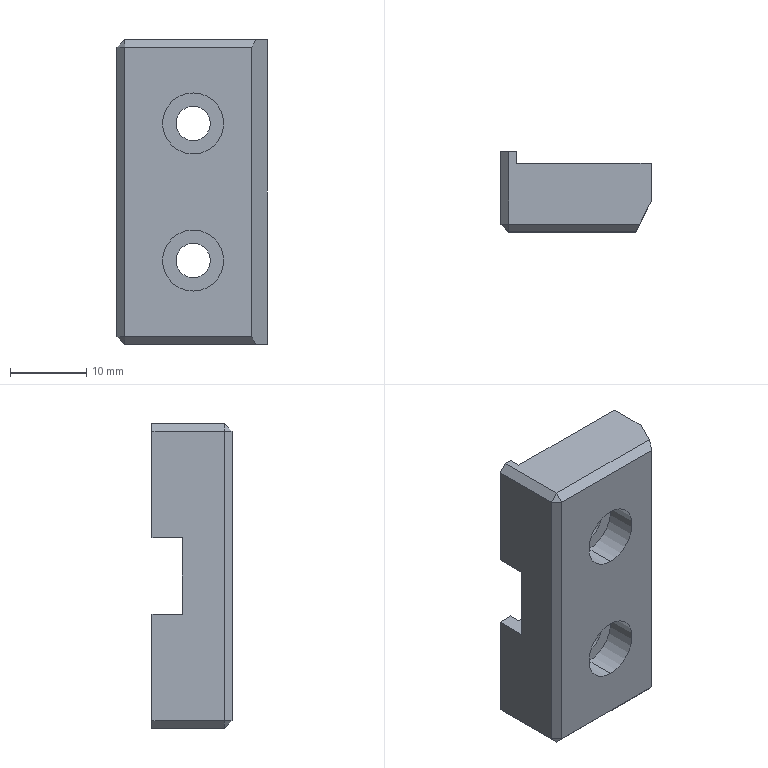Part | NX | features BREP 1 | 1 solid | 32 faces | box 19.7 x 10.5 x 40 mm | volume 5921 mm3 | plane 24 | cylinder 8 | commonest cylinder face diameters 4.5 x4 8 x4
STEP:
#1=CARTESIAN_POINT('',(-727.665,-5.,15.));
#2=VERTEX_POINT('',#1);
#3=CARTESIAN_POINT('',(-727.665,-5.,7.));
#4=VERTEX_POINT('',#3);
#5=CARTESIAN_POINT('',(-727.665,-5.,11.));
#6=DIRECTION('',(0.,-1.,0.));
#7=DIRECTION('',(0.,0.,-1.));
#8=AXIS2_PLACEMENT_3D('',#5,#6,#7);
#9=CIRCLE('',#8,4.);
#10=EDGE_CURVE('',#2,#4,#9,.T.);
#11=ORIENTED_EDGE('',*,*,#10,.F.);
#12=CARTESIAN_POINT('',(-727.665,-9.,15.));
#13=VERTEX_POINT('',#12);
#14=CARTESIAN_POINT('',(-727.665,-9.,15.));
#15=DIRECTION('',(0.,-1.,0.));
#16=VECTOR('',#15,1000.);
#17=LINE('',#14,#16);
#18=EDGE_CURVE('',#2,#13,#17,.T.);
#19=ORIENTED_EDGE('',*,*,#18,.T.);
#20=CARTESIAN_POINT('',(-727.665,-9.,7.));
#21=VERTEX_POINT('',#20);
#22=CARTESIAN_POINT('',(-727.665,-9.,11.));
#23=DIRECTION('',(0.,-1.,0.));
#24=DIRECTION('',(0.,0.,-1.));
#25=AXIS2_PLACEMENT_3D('',#22,#23,#24);
#26=CIRCLE('',#25,4.);
#27=EDGE_CURVE('',#13,#21,#26,.T.);
#28=ORIENTED_EDGE('',*,*,#27,.T.);
#29=CARTESIAN_POINT('',(-727.665,-9.,7.));
#30=DIRECTION('',(0.,-1.,0.));
#31=VECTOR('',#30,1000.);
#32=LINE('',#29,#31);
#33=EDGE_CURVE('',#4,#21,#32,.T.);
#34=ORIENTED_EDGE('',*,*,#33,.F.);
#35=EDGE_LOOP('',(#11,#19,#28,#34));
#36=FACE_BOUND('',#35,.T.);
#37=CARTESIAN_POINT('',(-727.665,-9.,11.));
#38=DIRECTION('',(0.,-1.,0.));
#39=DIRECTION('',(0.,0.,-1.));
#40=AXIS2_PLACEMENT_3D('',#37,#38,#39);
#41=CYLINDRICAL_SURFACE('',#40,4.);
#42=ADVANCED_FACE('',(#36),#41,.F.);
#43=CARTESIAN_POINT('',(-727.665,0.,13.25));
#44=VERTEX_POINT('',#43);
#45=CARTESIAN_POINT('',(-727.665,0.,8.75));
#46=VERTEX_POINT('',#45);
#47=CARTESIAN_POINT('',(-727.665,0.,11.));
#48=DIRECTION('',(0.,-1.,0.));
#49=DIRECTION('',(0.,0.,-1.));
#50=AXIS2_PLACEMENT_3D('',#47,#48,#49);
#51=CIRCLE('',#50,2.25);
#52=EDGE_CURVE('',#44,#46,#51,.T.);
#53=ORIENTED_EDGE('',*,*,#52,.F.);
#54=CARTESIAN_POINT('',(-727.665,-5.,13.25));
#55=VERTEX_POINT('',#54);
#56=CARTESIAN_POINT('',(-727.665,-9.,13.25));
#57=DIRECTION('',(0.,-1.,0.));
#58=VECTOR('',#57,1000.);
#59=LINE('',#56,#58);
#60=EDGE_CURVE('',#44,#55,#59,.T.);
#61=ORIENTED_EDGE('',*,*,#60,.T.);
#62=CARTESIAN_POINT('',(-727.665,-5.,8.75));
#63=VERTEX_POINT('',#62);
#64=CARTESIAN_POINT('',(-727.665,-5.,11.));
#65=DIRECTION('',(0.,-1.,0.));
#66=DIRECTION('',(0.,0.,-1.));
#67=AXIS2_PLACEMENT_3D('',#64,#65,#66);
#68=CIRCLE('',#67,2.25);
#69=EDGE_CURVE('',#55,#63,#68,.T.);
#70=ORIENTED_EDGE('',*,*,#69,.T.);
#71=CARTESIAN_POINT('',(-727.665,-9.,8.75));
#72=DIRECTION('',(0.,-1.,0.));
#73=VECTOR('',#72,1000.);
#74=LINE('',#71,#73);
#75=EDGE_CURVE('',#46,#63,#74,.T.);
#76=ORIENTED_EDGE('',*,*,#75,.F.);
#77=EDGE_LOOP('',(#53,#61,#70,#76));
#78=FACE_BOUND('',#77,.T.);
#79=CARTESIAN_POINT('',(-727.665,-9.,11.));
#80=DIRECTION('',(0.,-1.,0.));
#81=DIRECTION('',(0.,0.,-1.));
#82=AXIS2_PLACEMENT_3D('',#79,#80,#81);
#83=CYLINDRICAL_SURFACE('',#82,2.25);
#84=ADVANCED_FACE('',(#78),#83,.F.);
#85=CARTESIAN_POINT('',(-727.665,-5.,33.));
#86=VERTEX_POINT('',#85);
#87=CARTESIAN_POINT('',(-727.665,-5.,25.));
#88=VERTEX_POINT('',#87);
#89=CARTESIAN_POINT('',(-727.665,-5.,29.));
#90=DIRECTION('',(0.,-1.,0.));
#91=DIRECTION('',(0.,0.,-1.));
#92=AXIS2_PLACEMENT_3D('',#89,#90,#91);
#93=CIRCLE('',#92,4.);
#94=EDGE_CURVE('',#86,#88,#93,.T.);
#95=ORIENTED_EDGE('',*,*,#94,.F.);
#96=CARTESIAN_POINT('',(-727.665,-9.,33.));
#97=VERTEX_POINT('',#96);
#98=CARTESIAN_POINT('',(-727.665,-9.,33.));
#99=DIRECTION('',(0.,-1.,0.));
#100=VECTOR('',#99,1000.);
#101=LINE('',#98,#100);
#102=EDGE_CURVE('',#86,#97,#101,.T.);
#103=ORIENTED_EDGE('',*,*,#102,.T.);
#104=CARTESIAN_POINT('',(-727.665,-9.,25.));
#105=VERTEX_POINT('',#104);
#106=CARTESIAN_POINT('',(-727.665,-9.,29.));
#107=DIRECTION('',(0.,-1.,0.));
#108=DIRECTION('',(0.,0.,-1.));
#109=AXIS2_PLACEMENT_3D('',#106,#107,#108);
#110=CIRCLE('',#109,4.);
#111=EDGE_CURVE('',#97,#105,#110,.T.);
#112=ORIENTED_EDGE('',*,*,#111,.T.);
#113=CARTESIAN_POINT('',(-727.665,-9.,25.));
#114=DIRECTION('',(0.,-1.,0.));
#115=VECTOR('',#114,1000.);
#116=LINE('',#113,#115);
#117=EDGE_CURVE('',#88,#105,#116,.T.);
#118=ORIENTED_EDGE('',*,*,#117,.F.);
#119=EDGE_LOOP('',(#95,#103,#112,#118));
#120=FACE_BOUND('',#119,.T.);
#121=CARTESIAN_POINT('',(-727.665,-9.,29.));
#122=DIRECTION('',(0.,-1.,0.));
#123=DIRECTION('',(0.,0.,-1.));
#124=AXIS2_PLACEMENT_3D('',#121,#122,#123);
#125=CYLINDRICAL_SURFACE('',#124,4.);
#126=ADVANCED_FACE('',(#120),#125,.F.);
#127=CARTESIAN_POINT('',(-727.665,0.,31.25));
#128=VERTEX_POINT('',#127);
#129=CARTESIAN_POINT('',(-727.665,0.,26.75));
#130=VERTEX_POINT('',#129);
#131=CARTESIAN_POINT('',(-727.665,0.,29.));
#132=DIRECTION('',(0.,-1.,0.));
#133=DIRECTION('',(0.,0.,-1.));
#134=AXIS2_PLACEMENT_3D('',#131,#132,#133);
#135=CIRCLE('',#134,2.25);
#136=EDGE_CURVE('',#128,#130,#135,.T.);
#137=ORIENTED_EDGE('',*,*,#136,.F.);
#138=CARTESIAN_POINT('',(-727.665,-5.,31.25));
#139=VERTEX_POINT('',#138);
#140=CARTESIAN_POINT('',(-727.665,-9.,31.25));
#141=DIRECTION('',(0.,-1.,0.));
#142=VECTOR('',#141,1000.);
#143=LINE('',#140,#142);
#144=EDGE_CURVE('',#128,#139,#143,.T.);
#145=ORIENTED_EDGE('',*,*,#144,.T.);
#146=CARTESIAN_POINT('',(-727.665,-5.,26.75));
#147=VERTEX_POINT('',#146);
#148=CARTESIAN_POINT('',(-727.665,-5.,29.));
#149=DIRECTION('',(0.,-1.,0.));
#150=DIRECTION('',(0.,0.,-1.));
#151=AXIS2_PLACEMENT_3D('',#148,#149,#150);
#152=CIRCLE('',#151,2.25);
#153=EDGE_CURVE('',#139,#147,#152,.T.);
#154=ORIENTED_EDGE('',*,*,#153,.T.);
#155=CARTESIAN_POINT('',(-727.665,-9.,26.75));
#156=DIRECTION('',(0.,-1.,0.));
#157=VECTOR('',#156,1000.);
#158=LINE('',#155,#157);
#159=EDGE_CURVE('',#130,#147,#158,.T.);
#160=ORIENTED_EDGE('',*,*,#159,.F.);
#161=EDGE_LOOP('',(#137,#145,#154,#160));
#162=FACE_BOUND('',#161,.T.);
#163=CARTESIAN_POINT('',(-727.665,-9.,29.));
#164=DIRECTION('',(0.,-1.,0.));
#165=DIRECTION('',(0.,0.,-1.));
#166=AXIS2_PLACEMENT_3D('',#163,#164,#165);
#167=CYLINDRICAL_SURFACE('',#166,2.25);
#168=ADVANCED_FACE('',(#162),#167,.F.);
#169=CARTESIAN_POINT('',(-735.665,0.,0.));
#170=VERTEX_POINT('',#169);
#171=CARTESIAN_POINT('',(-735.665,0.,15.));
#172=VERTEX_POINT('',#171);
#173=CARTESIAN_POINT('',(-735.665,0.,-2.5));
#174=DIRECTION('',(0.,0.,1.));
#175=VECTOR('',#174,1000.);
#176=LINE('',#173,#175);
#177=EDGE_CURVE('',#170,#172,#176,.T.);
#178=ORIENTED_EDGE('',*,*,#177,.T.);
#179=CARTESIAN_POINT('',(-717.965,0.,15.));
#180=VERTEX_POINT('',#179);
#181=CARTESIAN_POINT('',(-737.665,0.,15.));
#182=DIRECTION('',(1.,0.,0.));
#183=VECTOR('',#182,1000.);
#184=LINE('',#181,#183);
#185=EDGE_CURVE('',#172,#180,#184,.T.);
#186=ORIENTED_EDGE('',*,*,#185,.T.);
#187=CARTESIAN_POINT('',(-717.965,0.,0.));
#188=VERTEX_POINT('',#187);
#189=CARTESIAN_POINT('',(-717.965,0.,40.));
#190=DIRECTION('',(0.,0.,-1.));
#191=VECTOR('',#190,1000.);
#192=LINE('',#189,#191);
#193=EDGE_CURVE('',#180,#188,#192,.T.);
#194=ORIENTED_EDGE('',*,*,#193,.T.);
#195=CARTESIAN_POINT('',(-737.665,0.,0.));
#196=DIRECTION('',(-1.,0.,0.));
#197=VECTOR('',#196,1000.);
#198=LINE('',#195,#197);
#199=EDGE_CURVE('',#188,#170,#198,.T.);
#200=ORIENTED_EDGE('',*,*,#199,.T.);
#201=EDGE_LOOP('',(#178,#186,#194,#200));
#202=FACE_BOUND('',#201,.T.);
#203=CARTESIAN_POINT('',(-727.665,0.,11.));
#204=DIRECTION('',(0.,-1.,0.));
#205=DIRECTION('',(0.,0.,-1.));
#206=AXIS2_PLACEMENT_3D('',#203,#204,#205);
#207=CIRCLE('',#206,2.25);
#208=EDGE_CURVE('',#46,#44,#207,.T.);
#209=ORIENTED_EDGE('',*,*,#208,.T.);
#210=ORIENTED_EDGE('',*,*,#52,.T.);
#211=EDGE_LOOP('',(#209,#210));
#212=FACE_BOUND('',#211,.T.);
#213=CARTESIAN_POINT('',(-737.665,0.,40.));
#214=DIRECTION('',(0.,-1.,0.));
#215=DIRECTION('',(0.,0.,-1.));
#216=AXIS2_PLACEMENT_3D('',#213,#214,#215);
#217=PLANE('',#216);
#218=ADVANCED_FACE('',(#202,#212),#217,.F.);
#219=CARTESIAN_POINT('',(-736.665,1.5,0.));
#220=VERTEX_POINT('',#219);
#221=CARTESIAN_POINT('',(-735.665,1.5,0.));
#222=VERTEX_POINT('',#221);
#223=CARTESIAN_POINT('',(-737.665,1.5,0.));
#224=DIRECTION('',(1.,0.,0.));
#225=VECTOR('',#224,1000.);
#226=LINE('',#223,#225);
#227=EDGE_CURVE('',#220,#222,#226,.T.);
#228=ORIENTED_EDGE('',*,*,#227,.F.);
#229=CARTESIAN_POINT('',(-737.665,1.5,1.));
#230=VERTEX_POINT('',#229);
#231=CARTESIAN_POINT('',(-735.915,1.5,-0.75));
#232=DIRECTION('',(-0.7071,0.,0.7071));
#233=VECTOR('',#232,1000.);
#234=LINE('',#231,#233);
#235=EDGE_CURVE('',#220,#230,#234,.T.);
#236=ORIENTED_EDGE('',*,*,#235,.T.);
#237=CARTESIAN_POINT('',(-737.665,1.5,15.));
#238=VERTEX_POINT('',#237);
#239=CARTESIAN_POINT('',(-737.665,1.5,-2.5));
#240=DIRECTION('',(0.,0.,1.));
#241=VECTOR('',#240,1000.);
#242=LINE('',#239,#241);
#243=EDGE_CURVE('',#230,#238,#242,.T.);
#244=ORIENTED_EDGE('',*,*,#243,.T.);
#245=CARTESIAN_POINT('',(-735.665,1.5,15.));
#246=VERTEX_POINT('',#245);
#247=CARTESIAN_POINT('',(-737.665,1.5,15.));
#248=DIRECTION('',(-1.,0.,0.));
#249=VECTOR('',#248,1000.);
#250=LINE('',#247,#249);
#251=EDGE_CURVE('',#246,#238,#250,.T.);
#252=ORIENTED_EDGE('',*,*,#251,.F.);
#253=CARTESIAN_POINT('',(-735.665,1.5,-2.5));
#254=DIRECTION('',(0.,0.,1.));
#255=VECTOR('',#254,1000.);
#256=LINE('',#253,#255);
#257=EDGE_CURVE('',#222,#246,#256,.T.);
#258=ORIENTED_EDGE('',*,*,#257,.F.);
#259=EDGE_LOOP('',(#228,#236,#244,#252,#258));
#260=FACE_BOUND('',#259,.T.);
#261=CARTESIAN_POINT('',(-737.665,1.5,-2.5));
#262=DIRECTION('',(0.,1.,0.));
#263=DIRECTION('',(1.,0.,0.));
#264=AXIS2_PLACEMENT_3D('',#261,#262,#263);
#265=PLANE('',#264);
#266=ADVANCED_FACE('',(#260),#265,.T.);
#267=CARTESIAN_POINT('',(-735.665,0.,15.));
#268=DIRECTION('',(0.,1.,0.));
#269=VECTOR('',#268,1000.);
#270=LINE('',#267,#269);
#271=EDGE_CURVE('',#172,#246,#270,.T.);
#272=ORIENTED_EDGE('',*,*,#271,.F.);
#273=ORIENTED_EDGE('',*,*,#177,.F.);
#274=CARTESIAN_POINT('',(-735.665,0.,0.));
#275=DIRECTION('',(0.,-1.,0.));
#276=VECTOR('',#275,1000.);
#277=LINE('',#274,#276);
#278=EDGE_CURVE('',#222,#170,#277,.T.);
#279=ORIENTED_EDGE('',*,*,#278,.F.);
#280=ORIENTED_EDGE('',*,*,#257,.T.);
#281=EDGE_LOOP('',(#272,#273,#279,#280));
#282=FACE_BOUND('',#281,.T.);
#283=CARTESIAN_POINT('',(-735.665,0.,-2.5));
#284=DIRECTION('',(1.,0.,0.));
#285=DIRECTION('',(0.,1.,0.));
#286=AXIS2_PLACEMENT_3D('',#283,#284,#285);
#287=PLANE('',#286);
#288=ADVANCED_FACE('',(#282),#287,.T.);
#289=CARTESIAN_POINT('',(-737.665,-8.,1.));
#290=VERTEX_POINT('',#289);
#291=CARTESIAN_POINT('',(-737.665,-8.,39.));
#292=VERTEX_POINT('',#291);
#293=CARTESIAN_POINT('',(-737.665,-8.,40.));
#294=DIRECTION('',(0.,0.,1.));
#295=VECTOR('',#294,1000.);
#296=LINE('',#293,#295);
#297=EDGE_CURVE('',#290,#292,#296,.T.);
#298=ORIENTED_EDGE('',*,*,#297,.T.);
#299=CARTESIAN_POINT('',(-737.665,1.5,39.));
#300=VERTEX_POINT('',#299);
#301=CARTESIAN_POINT('',(-737.665,1.5,39.));
#302=DIRECTION('',(0.,1.,0.));
#303=VECTOR('',#302,1000.);
#304=LINE('',#301,#303);
#305=EDGE_CURVE('',#292,#300,#304,.T.);
#306=ORIENTED_EDGE('',*,*,#305,.T.);
#307=CARTESIAN_POINT('',(-737.665,1.5,25.));
#308=VERTEX_POINT('',#307);
#309=CARTESIAN_POINT('',(-737.665,1.5,-2.5));
#310=DIRECTION('',(0.,0.,1.));
#311=VECTOR('',#310,1000.);
#312=LINE('',#309,#311);
#313=EDGE_CURVE('',#308,#300,#312,.T.);
#314=ORIENTED_EDGE('',*,*,#313,.F.);
#315=CARTESIAN_POINT('',(-737.665,-2.5,25.));
#316=VERTEX_POINT('',#315);
#317=CARTESIAN_POINT('',(-737.665,-2.5,25.));
#318=DIRECTION('',(0.,1.,0.));
#319=VECTOR('',#318,1000.);
#320=LINE('',#317,#319);
#321=EDGE_CURVE('',#316,#308,#320,.T.);
#322=ORIENTED_EDGE('',*,*,#321,.F.);
#323=CARTESIAN_POINT('',(-737.665,-2.5,15.));
#324=VERTEX_POINT('',#323);
#325=CARTESIAN_POINT('',(-737.665,-2.5,25.));
#326=DIRECTION('',(0.,0.,1.));
#327=VECTOR('',#326,1000.);
#328=LINE('',#325,#327);
#329=EDGE_CURVE('',#324,#316,#328,.T.);
#330=ORIENTED_EDGE('',*,*,#329,.F.);
#331=CARTESIAN_POINT('',(-737.665,-2.5,15.));
#332=DIRECTION('',(0.,1.,0.));
#333=VECTOR('',#332,1000.);
#334=LINE('',#331,#333);
#335=EDGE_CURVE('',#324,#238,#334,.T.);
#336=ORIENTED_EDGE('',*,*,#335,.T.);
#337=ORIENTED_EDGE('',*,*,#243,.F.);
#338=CARTESIAN_POINT('',(-737.665,0.,1.));
#339=DIRECTION('',(0.,-1.,0.));
#340=VECTOR('',#339,1000.);
#341=LINE('',#338,#340);
#342=EDGE_CURVE('',#230,#290,#341,.T.);
#343=ORIENTED_EDGE('',*,*,#342,.T.);
#344=EDGE_LOOP('',(#298,#306,#314,#322,#330,#336,#337,#343));
#345=FACE_BOUND('',#344,.T.);
#346=CARTESIAN_POINT('',(-737.665,0.,40.));
#347=DIRECTION('',(1.,0.,0.));
#348=DIRECTION('',(0.,1.,0.));
#349=AXIS2_PLACEMENT_3D('',#346,#347,#348);
#350=PLANE('',#349);
#351=ADVANCED_FACE('',(#345),#350,.F.);
#352=CARTESIAN_POINT('',(-736.665,-9.,39.));
#353=VERTEX_POINT('',#352);
#354=CARTESIAN_POINT('',(-736.665,-9.,1.));
#355=VERTEX_POINT('',#354);
#356=CARTESIAN_POINT('',(-736.665,-9.,40.));
#357=DIRECTION('',(0.,0.,-1.));
#358=VECTOR('',#357,1000.);
#359=LINE('',#356,#358);
#360=EDGE_CURVE('',#353,#355,#359,.T.);
#361=ORIENTED_EDGE('',*,*,#360,.T.);
#362=CARTESIAN_POINT('',(-719.965,-9.,1.));
#363=VERTEX_POINT('',#362);
#364=CARTESIAN_POINT('',(-737.665,-9.,1.));
#365=DIRECTION('',(1.,0.,0.));
#366=VECTOR('',#365,1000.);
#367=LINE('',#364,#366);
#368=EDGE_CURVE('',#355,#363,#367,.T.);
#369=ORIENTED_EDGE('',*,*,#368,.T.);
#370=CARTESIAN_POINT('',(-719.965,-9.,39.));
#371=VERTEX_POINT('',#370);
#372=CARTESIAN_POINT('',(-719.965,-9.,40.));
#373=DIRECTION('',(0.,0.,1.));
#374=VECTOR('',#373,1000.);
#375=LINE('',#372,#374);
#376=EDGE_CURVE('',#363,#371,#375,.T.);
#377=ORIENTED_EDGE('',*,*,#376,.T.);
#378=CARTESIAN_POINT('',(-737.665,-9.,39.));
#379=DIRECTION('',(-1.,0.,0.));
#380=VECTOR('',#379,1000.);
#381=LINE('',#378,#380);
#382=EDGE_CURVE('',#371,#353,#381,.T.);
#383=ORIENTED_EDGE('',*,*,#382,.T.);
#384=EDGE_LOOP('',(#361,#369,#377,#383));
#385=FACE_BOUND('',#384,.T.);
#386=CARTESIAN_POINT('',(-727.665,-9.,11.));
#387=DIRECTION('',(0.,-1.,0.));
#388=DIRECTION('',(0.,0.,-1.));
#389=AXIS2_PLACEMENT_3D('',#386,#387,#388);
#390=CIRCLE('',#389,4.);
#391=EDGE_CURVE('',#21,#13,#390,.T.);
#392=ORIENTED_EDGE('',*,*,#391,.F.);
#393=ORIENTED_EDGE('',*,*,#27,.F.);
#394=EDGE_LOOP('',(#392,#393));
#395=FACE_BOUND('',#394,.T.);
#396=CARTESIAN_POINT('',(-727.665,-9.,29.));
#397=DIRECTION('',(0.,-1.,0.));
#398=DIRECTION('',(0.,0.,-1.));
#399=AXIS2_PLACEMENT_3D('',#396,#397,#398);
#400=CIRCLE('',#399,4.);
#401=EDGE_CURVE('',#105,#97,#400,.T.);
#402=ORIENTED_EDGE('',*,*,#401,.F.);
#403=ORIENTED_EDGE('',*,*,#111,.F.);
#404=EDGE_LOOP('',(#402,#403));
#405=FACE_BOUND('',#404,.T.);
#406=CARTESIAN_POINT('',(-737.665,-9.,40.));
#407=DIRECTION('',(0.,1.,0.));
#408=DIRECTION('',(1.,0.,0.));
#409=AXIS2_PLACEMENT_3D('',#406,#407,#408);
#410=PLANE('',#409);
#411=ADVANCED_FACE('',(#385,#395,#405),#410,.F.);
#412=ORIENTED_EDGE('',*,*,#193,.F.);
#413=CARTESIAN_POINT('',(-717.965,-2.5,15.));
#414=VERTEX_POINT('',#413);
#415=CARTESIAN_POINT('',(-717.965,-2.5,15.));
#416=DIRECTION('',(0.,1.,0.));
#417=VECTOR('',#416,1000.);
#418=LINE('',#415,#417);
#419=EDGE_CURVE('',#414,#180,#418,.T.);
#420=ORIENTED_EDGE('',*,*,#419,.F.);
#421=CARTESIAN_POINT('',(-717.965,-2.5,25.));
#422=VERTEX_POINT('',#421);
#423=CARTESIAN_POINT('',(-717.965,-2.5,25.));
#424=DIRECTION('',(0.,0.,-1.));
#425=VECTOR('',#424,1000.);
#426=LINE('',#423,#425);
#427=EDGE_CURVE('',#422,#414,#426,.T.);
#428=ORIENTED_EDGE('',*,*,#427,.F.);
#429=CARTESIAN_POINT('',(-717.965,0.,25.));
#430=VERTEX_POINT('',#429);
#431=CARTESIAN_POINT('',(-717.965,-2.5,25.));
#432=DIRECTION('',(0.,1.,0.));
#433=VECTOR('',#432,1000.);
#434=LINE('',#431,#433);
#435=EDGE_CURVE('',#422,#430,#434,.T.);
#436=ORIENTED_EDGE('',*,*,#435,.T.);
#437=CARTESIAN_POINT('',(-717.965,0.,40.));
#438=VERTEX_POINT('',#437);
#439=CARTESIAN_POINT('',(-717.965,0.,40.));
#440=DIRECTION('',(0.,0.,-1.));
#441=VECTOR('',#440,1000.);
#442=LINE('',#439,#441);
#443=EDGE_CURVE('',#438,#430,#442,.T.);
#444=ORIENTED_EDGE('',*,*,#443,.F.);
#445=CARTESIAN_POINT('',(-717.965,-5.,40.));
#446=VERTEX_POINT('',#445);
#447=CARTESIAN_POINT('',(-717.965,0.,40.));
#448=DIRECTION('',(0.,1.,0.));
#449=VECTOR('',#448,1000.);
#450=LINE('',#447,#449);
#451=EDGE_CURVE('',#446,#438,#450,.T.);
#452=ORIENTED_EDGE('',*,*,#451,.F.);
#453=CARTESIAN_POINT('',(-717.965,-5.,0.));
#454=VERTEX_POINT('',#453);
#455=CARTESIAN_POINT('',(-717.965,-5.,40.));
#456=DIRECTION('',(0.,0.,-1.));
#457=VECTOR('',#456,1000.);
#458=LINE('',#455,#457);
#459=EDGE_CURVE('',#446,#454,#458,.T.);
#460=ORIENTED_EDGE('',*,*,#459,.T.);
#461=CARTESIAN_POINT('',(-717.965,0.,0.));
#462=DIRECTION('',(0.,1.,0.));
#463=VECTOR('',#462,1000.);
#464=LINE('',#461,#463);
#465=EDGE_CURVE('',#454,#188,#464,.T.);
#466=ORIENTED_EDGE('',*,*,#465,.T.);
#467=EDGE_LOOP('',(#412,#420,#428,#436,#444,#452,#460,#466));
#468=FACE_BOUND('',#467,.T.);
#469=CARTESIAN_POINT('',(-717.965,0.,40.));
#470=DIRECTION('',(-1.,0.,0.));
#471=DIRECTION('',(0.,0.,1.));
#472=AXIS2_PLACEMENT_3D('',#469,#470,#471);
#473=PLANE('',#472);
#474=ADVANCED_FACE('',(#468),#473,.F.);
#475=ORIENTED_EDGE('',*,*,#443,.T.);
#476=CARTESIAN_POINT('',(-735.665,0.,25.));
#477=VERTEX_POINT('',#476);
#478=CARTESIAN_POINT('',(-737.665,0.,25.));
#479=DIRECTION('',(-1.,0.,0.));
#480=VECTOR('',#479,1000.);
#481=LINE('',#478,#480);
#482=EDGE_CURVE('',#430,#477,#481,.T.);
#483=ORIENTED_EDGE('',*,*,#482,.T.);
#484=CARTESIAN_POINT('',(-735.665,0.,40.));
#485=VERTEX_POINT('',#484);
#486=CARTESIAN_POINT('',(-735.665,0.,-2.5));
#487=DIRECTION('',(0.,0.,1.));
#488=VECTOR('',#487,1000.);
#489=LINE('',#486,#488);
#490=EDGE_CURVE('',#477,#485,#489,.T.);
#491=ORIENTED_EDGE('',*,*,#490,.T.);
#492=CARTESIAN_POINT('',(-737.665,0.,40.));
#493=DIRECTION('',(-1.,0.,0.));
#494=VECTOR('',#493,1000.);
#495=LINE('',#492,#494);
#496=EDGE_CURVE('',#438,#485,#495,.T.);
#497=ORIENTED_EDGE('',*,*,#496,.F.);
#498=EDGE_LOOP('',(#475,#483,#491,#497));
#499=FACE_BOUND('',#498,.T.);
#500=CARTESIAN_POINT('',(-727.665,0.,29.));
#501=DIRECTION('',(0.,-1.,0.));
#502=DIRECTION('',(0.,0.,-1.));
#503=AXIS2_PLACEMENT_3D('',#500,#501,#502);
#504=CIRCLE('',#503,2.25);
#505=EDGE_CURVE('',#130,#128,#504,.T.);
#506=ORIENTED_EDGE('',*,*,#505,.T.);
#507=ORIENTED_EDGE('',*,*,#136,.T.);
#508=EDGE_LOOP('',(#506,#507));
#509=FACE_BOUND('',#508,.T.);
#510=CARTESIAN_POINT('',(-737.665,0.,40.));
#511=DIRECTION('',(0.,-1.,0.));
#512=DIRECTION('',(0.,0.,-1.));
#513=AXIS2_PLACEMENT_3D('',#510,#511,#512);
#514=PLANE('',#513);
#515=ADVANCED_FACE('',(#499,#509),#514,.F.);
#516=CARTESIAN_POINT('',(-735.665,1.5,40.));
#517=VERTEX_POINT('',#516);
#518=CARTESIAN_POINT('',(-736.665,1.5,40.));
#519=VERTEX_POINT('',#518);
#520=CARTESIAN_POINT('',(-737.665,1.5,40.));
#521=DIRECTION('',(-1.,0.,0.));
#522=VECTOR('',#521,1000.);
#523=LINE('',#520,#522);
#524=EDGE_CURVE('',#517,#519,#523,.T.);
#525=ORIENTED_EDGE('',*,*,#524,.T.);
#526=CARTESIAN_POINT('',(-736.665,-8.,40.));
#527=VERTEX_POINT('',#526);
#528=CARTESIAN_POINT('',(-736.665,-9.,40.));
#529=DIRECTION('',(0.,-1.,0.));
#530=VECTOR('',#529,1000.);
#531=LINE('',#528,#530);
#532=EDGE_CURVE('',#519,#527,#531,.T.);
#533=ORIENTED_EDGE('',*,*,#532,.T.);
#534=CARTESIAN_POINT('',(-719.465,-8.,40.));
#535=VERTEX_POINT('',#534);
#536=CARTESIAN_POINT('',(-719.965,-8.,40.));
#537=DIRECTION('',(1.,0.,0.));
#538=VECTOR('',#537,1000.);
#539=LINE('',#536,#538);
#540=EDGE_CURVE('',#527,#535,#539,.T.);
#541=ORIENTED_EDGE('',*,*,#540,.T.);
#542=CARTESIAN_POINT('',(-723.505,-16.08,40.));
#543=DIRECTION('',(0.4472,0.8944,0.));
#544=VECTOR('',#543,1000.);
#545=LINE('',#542,#544);
#546=EDGE_CURVE('',#535,#446,#545,.T.);
#547=ORIENTED_EDGE('',*,*,#546,.T.);
#548=ORIENTED_EDGE('',*,*,#451,.T.);
#549=ORIENTED_EDGE('',*,*,#496,.T.);
#550=CARTESIAN_POINT('',(-735.665,0.,40.));
#551=DIRECTION('',(0.,1.,0.));
#552=VECTOR('',#551,1000.);
#553=LINE('',#550,#552);
#554=EDGE_CURVE('',#485,#517,#553,.T.);
#555=ORIENTED_EDGE('',*,*,#554,.T.);
#556=EDGE_LOOP('',(#525,#533,#541,#547,#548,#549,#555));
#557=FACE_BOUND('',#556,.T.);
#558=CARTESIAN_POINT('',(-737.665,-9.,40.));
#559=DIRECTION('',(0.,0.,1.));
#560=DIRECTION('',(1.,0.,0.));
#561=AXIS2_PLACEMENT_3D('',#558,#559,#560);
#562=PLANE('',#561);
#563=ADVANCED_FACE('',(#557),#562,.T.);
#564=CARTESIAN_POINT('',(-719.465,-8.,0.));
#565=VERTEX_POINT('',#564);
#566=CARTESIAN_POINT('',(-736.665,-8.,0.));
#567=VERTEX_POINT('',#566);
#568=CARTESIAN_POINT('',(-737.665,-8.,0.));
#569=DIRECTION('',(-1.,0.,0.));
#570=VECTOR('',#569,1000.);
#571=LINE('',#568,#570);
#572=EDGE_CURVE('',#565,#567,#571,.T.);
#573=ORIENTED_EDGE('',*,*,#572,.T.);
#574=CARTESIAN_POINT('',(-736.665,-9.,0.));
#575=DIRECTION('',(0.,1.,0.));
#576=VECTOR('',#575,1000.);
#577=LINE('',#574,#576);
#578=EDGE_CURVE('',#567,#220,#577,.T.);
#579=ORIENTED_EDGE('',*,*,#578,.T.);
#580=ORIENTED_EDGE('',*,*,#227,.T.);
#581=ORIENTED_EDGE('',*,*,#278,.T.);
#582=ORIENTED_EDGE('',*,*,#199,.F.);
#583=ORIENTED_EDGE('',*,*,#465,.F.);
#584=CARTESIAN_POINT('',(-717.965,-5.,0.));
#585=DIRECTION('',(-0.4472,-0.8944,0.));
#586=VECTOR('',#585,1000.);
#587=LINE('',#584,#586);
#588=EDGE_CURVE('',#454,#565,#587,.T.);
#589=ORIENTED_EDGE('',*,*,#588,.T.);
#590=EDGE_LOOP('',(#573,#579,#580,#581,#582,#583,#589));
#591=FACE_BOUND('',#590,.T.);
#592=CARTESIAN_POINT('',(-737.665,-9.,0.));
#593=DIRECTION('',(0.,0.,1.));
#594=DIRECTION('',(1.,0.,0.));
#595=AXIS2_PLACEMENT_3D('',#592,#593,#594);
#596=PLANE('',#595);
#597=ADVANCED_FACE('',(#591),#596,.F.);
#598=ORIENTED_EDGE('',*,*,#313,.T.);
#599=CARTESIAN_POINT('',(-758.415,1.5,18.25));
#600=DIRECTION('',(0.7071,0.,0.7071));
#601=VECTOR('',#600,1000.);
#602=LINE('',#599,#601);
#603=EDGE_CURVE('',#300,#519,#602,.T.);
#604=ORIENTED_EDGE('',*,*,#603,.T.);
#605=ORIENTED_EDGE('',*,*,#524,.F.);
#606=CARTESIAN_POINT('',(-735.665,1.5,25.));
#607=VERTEX_POINT('',#606);
#608=CARTESIAN_POINT('',(-735.665,1.5,-2.5));
#609=DIRECTION('',(0.,0.,1.));
#610=VECTOR('',#609,1000.);
#611=LINE('',#608,#610);
#612=EDGE_CURVE('',#607,#517,#611,.T.);
#613=ORIENTED_EDGE('',*,*,#612,.F.);
#614=CARTESIAN_POINT('',(-737.665,1.5,25.));
#615=DIRECTION('',(1.,0.,0.));
#616=VECTOR('',#615,1000.);
#617=LINE('',#614,#616);
#618=EDGE_CURVE('',#308,#607,#617,.T.);
#619=ORIENTED_EDGE('',*,*,#618,.F.);
#620=EDGE_LOOP('',(#598,#604,#605,#613,#619));
#621=FACE_BOUND('',#620,.T.);
#622=CARTESIAN_POINT('',(-737.665,1.5,-2.5));
#623=DIRECTION('',(0.,1.,0.));
#624=DIRECTION('',(1.,0.,0.));
#625=AXIS2_PLACEMENT_3D('',#622,#623,#624);
#626=PLANE('',#625);
#627=ADVANCED_FACE('',(#621),#626,.T.);
#628=CARTESIAN_POINT('',(-735.665,0.,25.));
#629=DIRECTION('',(0.,-1.,0.));
#630=VECTOR('',#629,1000.);
#631=LINE('',#628,#630);
#632=EDGE_CURVE('',#607,#477,#631,.T.);
#633=ORIENTED_EDGE('',*,*,#632,.F.);
#634=ORIENTED_EDGE('',*,*,#612,.T.);
#635=ORIENTED_EDGE('',*,*,#554,.F.);
#636=ORIENTED_EDGE('',*,*,#490,.F.);
#637=EDGE_LOOP('',(#633,#634,#635,#636));
#638=FACE_BOUND('',#637,.T.);
#639=CARTESIAN_POINT('',(-735.665,0.,-2.5));
#640=DIRECTION('',(1.,0.,0.));
#641=DIRECTION('',(0.,1.,0.));
#642=AXIS2_PLACEMENT_3D('',#639,#640,#641);
#643=PLANE('',#642);
#644=ADVANCED_FACE('',(#638),#643,.T.);
#645=ORIENTED_EDGE('',*,*,#144,.F.);
#646=ORIENTED_EDGE('',*,*,#505,.F.);
#647=ORIENTED_EDGE('',*,*,#159,.T.);
#648=CARTESIAN_POINT('',(-727.665,-5.,29.));
#649=DIRECTION('',(0.,-1.,0.));
#650=DIRECTION('',(0.,0.,-1.));
#651=AXIS2_PLACEMENT_3D('',#648,#649,#650);
#652=CIRCLE('',#651,2.25);
#653=EDGE_CURVE('',#147,#139,#652,.T.);
#654=ORIENTED_EDGE('',*,*,#653,.T.);
#655=EDGE_LOOP('',(#645,#646,#647,#654));
#656=FACE_BOUND('',#655,.T.);
#657=CARTESIAN_POINT('',(-727.665,-9.,29.));
#658=DIRECTION('',(0.,-1.,0.));
#659=DIRECTION('',(0.,0.,-1.));
#660=AXIS2_PLACEMENT_3D('',#657,#658,#659);
#661=CYLINDRICAL_SURFACE('',#660,2.25);
#662=ADVANCED_FACE('',(#656),#661,.F.);
#663=CARTESIAN_POINT('',(-727.665,-5.,29.));
#664=DIRECTION('',(0.,-1.,0.));
#665=DIRECTION('',(0.,0.,-1.));
#666=AXIS2_PLACEMENT_3D('',#663,#664,#665);
#667=CIRCLE('',#666,4.);
#668=EDGE_CURVE('',#88,#86,#667,.T.);
#669=ORIENTED_EDGE('',*,*,#668,.T.);
#670=ORIENTED_EDGE('',*,*,#94,.T.);
#671=EDGE_LOOP('',(#669,#670));
#672=FACE_BOUND('',#671,.T.);
#673=ORIENTED_EDGE('',*,*,#653,.F.);
#674=ORIENTED_EDGE('',*,*,#153,.F.);
#675=EDGE_LOOP('',(#673,#674));
#676=FACE_BOUND('',#675,.T.);
#677=CARTESIAN_POINT('',(-725.415,-5.,29.));
#678=DIRECTION('',(0.,1.,0.));
#679=DIRECTION('',(1.,0.,0.));
#680=AXIS2_PLACEMENT_3D('',#677,#678,#679);
#681=PLANE('',#680);
#682=ADVANCED_FACE('',(#672,#676),#681,.F.);
#683=ORIENTED_EDGE('',*,*,#102,.F.);
#684=ORIENTED_EDGE('',*,*,#668,.F.);
#685=ORIENTED_EDGE('',*,*,#117,.T.);
#686=ORIENTED_EDGE('',*,*,#401,.T.);
#687=EDGE_LOOP('',(#683,#684,#685,#686));
#688=FACE_BOUND('',#687,.T.);
#689=CARTESIAN_POINT('',(-727.665,-9.,29.));
#690=DIRECTION('',(0.,-1.,0.));
#691=DIRECTION('',(0.,0.,-1.));
#692=AXIS2_PLACEMENT_3D('',#689,#690,#691);
#693=CYLINDRICAL_SURFACE('',#692,4.);
#694=ADVANCED_FACE('',(#688),#693,.F.);
#695=ORIENTED_EDGE('',*,*,#60,.F.);
#696=ORIENTED_EDGE('',*,*,#208,.F.);
#697=ORIENTED_EDGE('',*,*,#75,.T.);
#698=CARTESIAN_POINT('',(-727.665,-5.,11.));
#699=DIRECTION('',(0.,-1.,0.));
#700=DIRECTION('',(0.,0.,-1.));
#701=AXIS2_PLACEMENT_3D('',#698,#699,#700);
#702=CIRCLE('',#701,2.25);
#703=EDGE_CURVE('',#63,#55,#702,.T.);
#704=ORIENTED_EDGE('',*,*,#703,.T.);
#705=EDGE_LOOP('',(#695,#696,#697,#704));
#706=FACE_BOUND('',#705,.T.);
#707=CARTESIAN_POINT('',(-727.665,-9.,11.));
#708=DIRECTION('',(0.,-1.,0.));
#709=DIRECTION('',(0.,0.,-1.));
#710=AXIS2_PLACEMENT_3D('',#707,#708,#709);
#711=CYLINDRICAL_SURFACE('',#710,2.25);
#712=ADVANCED_FACE('',(#706),#711,.F.);
#713=CARTESIAN_POINT('',(-727.665,-5.,11.));
#714=DIRECTION('',(0.,-1.,0.));
#715=DIRECTION('',(0.,0.,-1.));
#716=AXIS2_PLACEMENT_3D('',#713,#714,#715);
#717=CIRCLE('',#716,4.);
#718=EDGE_CURVE('',#4,#2,#717,.T.);
#719=ORIENTED_EDGE('',*,*,#718,.T.);
#720=ORIENTED_EDGE('',*,*,#10,.T.);
#721=EDGE_LOOP('',(#719,#720));
#722=FACE_BOUND('',#721,.T.);
#723=ORIENTED_EDGE('',*,*,#703,.F.);
#724=ORIENTED_EDGE('',*,*,#69,.F.);
#725=EDGE_LOOP('',(#723,#724));
#726=FACE_BOUND('',#725,.T.);
#727=CARTESIAN_POINT('',(-725.415,-5.,11.));
#728=DIRECTION('',(0.,1.,0.));
#729=DIRECTION('',(1.,0.,0.));
#730=AXIS2_PLACEMENT_3D('',#727,#728,#729);
#731=PLANE('',#730);
#732=ADVANCED_FACE('',(#722,#726),#731,.F.);
#733=ORIENTED_EDGE('',*,*,#18,.F.);
#734=ORIENTED_EDGE('',*,*,#718,.F.);
#735=ORIENTED_EDGE('',*,*,#33,.T.);
#736=ORIENTED_EDGE('',*,*,#391,.T.);
#737=EDGE_LOOP('',(#733,#734,#735,#736));
#738=FACE_BOUND('',#737,.T.);
#739=CARTESIAN_POINT('',(-727.665,-9.,11.));
#740=DIRECTION('',(0.,-1.,0.));
#741=DIRECTION('',(0.,0.,-1.));
#742=AXIS2_PLACEMENT_3D('',#739,#740,#741);
#743=CYLINDRICAL_SURFACE('',#742,4.);
#744=ADVANCED_FACE('',(#738),#743,.F.);
#745=ORIENTED_EDGE('',*,*,#376,.F.);
#746=CARTESIAN_POINT('',(-727.521,-24.111,16.111));
#747=DIRECTION('',(0.3333,0.6667,-0.6667));
#748=VECTOR('',#747,1000.);
#749=LINE('',#746,#748);
#750=EDGE_CURVE('',#363,#565,#749,.T.);
#751=ORIENTED_EDGE('',*,*,#750,.T.);
#752=ORIENTED_EDGE('',*,*,#588,.F.);
#753=ORIENTED_EDGE('',*,*,#459,.F.);
#754=ORIENTED_EDGE('',*,*,#546,.F.);
#755=CARTESIAN_POINT('',(-718.632,-6.333,41.667));
#756=DIRECTION('',(-0.3333,-0.6667,-0.6667));
#757=VECTOR('',#756,1000.);
#758=LINE('',#755,#757);
#759=EDGE_CURVE('',#535,#371,#758,.T.);
#760=ORIENTED_EDGE('',*,*,#759,.T.);
#761=EDGE_LOOP('',(#745,#751,#752,#753,#754,#760));
#762=FACE_BOUND('',#761,.T.);
#763=CARTESIAN_POINT('',(-717.965,-5.,40.));
#764=DIRECTION('',(-0.8944,0.4472,0.));
#765=DIRECTION('',(0.,0.,1.));
#766=AXIS2_PLACEMENT_3D('',#763,#764,#765);
#767=PLANE('',#766);
#768=ADVANCED_FACE('',(#762),#767,.F.);
#769=ORIENTED_EDGE('',*,*,#271,.T.);
#770=ORIENTED_EDGE('',*,*,#251,.T.);
#771=ORIENTED_EDGE('',*,*,#335,.F.);
#772=CARTESIAN_POINT('',(-737.665,-2.5,15.));
#773=DIRECTION('',(-1.,0.,0.));
#774=VECTOR('',#773,1000.);
#775=LINE('',#772,#774);
#776=EDGE_CURVE('',#414,#324,#775,.T.);
#777=ORIENTED_EDGE('',*,*,#776,.F.);
#778=ORIENTED_EDGE('',*,*,#419,.T.);
#779=ORIENTED_EDGE('',*,*,#185,.F.);
#780=EDGE_LOOP('',(#769,#770,#771,#777,#778,#779));
#781=FACE_BOUND('',#780,.T.);
#782=CARTESIAN_POINT('',(-737.665,-2.5,15.));
#783=DIRECTION('',(0.,0.,-1.));
#784=DIRECTION('',(-1.,0.,0.));
#785=AXIS2_PLACEMENT_3D('',#782,#783,#784);
#786=PLANE('',#785);
#787=ADVANCED_FACE('',(#781),#786,.F.);
#788=ORIENTED_EDGE('',*,*,#435,.F.);
#789=CARTESIAN_POINT('',(-737.665,-2.5,25.));
#790=DIRECTION('',(1.,0.,0.));
#791=VECTOR('',#790,1000.);
#792=LINE('',#789,#791);
#793=EDGE_CURVE('',#316,#422,#792,.T.);
#794=ORIENTED_EDGE('',*,*,#793,.F.);
#795=ORIENTED_EDGE('',*,*,#321,.T.);
#796=ORIENTED_EDGE('',*,*,#618,.T.);
#797=ORIENTED_EDGE('',*,*,#632,.T.);
#798=ORIENTED_EDGE('',*,*,#482,.F.);
#799=EDGE_LOOP('',(#788,#794,#795,#796,#797,#798));
#800=FACE_BOUND('',#799,.T.);
#801=CARTESIAN_POINT('',(-737.665,-2.5,25.));
#802=DIRECTION('',(0.,0.,1.));
#803=DIRECTION('',(1.,0.,0.));
#804=AXIS2_PLACEMENT_3D('',#801,#802,#803);
#805=PLANE('',#804);
#806=ADVANCED_FACE('',(#800),#805,.F.);
#807=ORIENTED_EDGE('',*,*,#329,.T.);
#808=ORIENTED_EDGE('',*,*,#793,.T.);
#809=ORIENTED_EDGE('',*,*,#427,.T.);
#810=ORIENTED_EDGE('',*,*,#776,.T.);
#811=EDGE_LOOP('',(#807,#808,#809,#810));
#812=FACE_BOUND('',#811,.T.);
#813=CARTESIAN_POINT('',(-737.665,-2.5,15.));
#814=DIRECTION('',(0.,-1.,0.));
#815=DIRECTION('',(0.,0.,-1.));
#816=AXIS2_PLACEMENT_3D('',#813,#814,#815);
#817=PLANE('',#816);
#818=ADVANCED_FACE('',(#812),#817,.F.);
#819=ORIENTED_EDGE('',*,*,#750,.F.);
#820=ORIENTED_EDGE('',*,*,#368,.F.);
#821=CARTESIAN_POINT('',(-736.665,-8.5,0.5));
#822=DIRECTION('',(0.,-0.7071,0.7071));
#823=VECTOR('',#822,1000.);
#824=LINE('',#821,#823);
#825=EDGE_CURVE('',#567,#355,#824,.T.);
#826=ORIENTED_EDGE('',*,*,#825,.F.);
#827=ORIENTED_EDGE('',*,*,#572,.F.);
#828=EDGE_LOOP('',(#819,#820,#826,#827));
#829=FACE_BOUND('',#828,.T.);
#830=CARTESIAN_POINT('',(-737.665,-9.,1.));
#831=DIRECTION('',(0.,0.7071,0.7071));
#832=DIRECTION('',(1.,0.,0.));
#833=AXIS2_PLACEMENT_3D('',#830,#831,#832);
#834=PLANE('',#833);
#835=ADVANCED_FACE('',(#829),#834,.F.);
#836=ORIENTED_EDGE('',*,*,#235,.F.);
#837=ORIENTED_EDGE('',*,*,#578,.F.);
#838=CARTESIAN_POINT('',(-737.665,-8.,1.));
#839=DIRECTION('',(0.7071,0.,-0.7071));
#840=VECTOR('',#839,1000.);
#841=LINE('',#838,#840);
#842=EDGE_CURVE('',#290,#567,#841,.T.);
#843=ORIENTED_EDGE('',*,*,#842,.F.);
#844=ORIENTED_EDGE('',*,*,#342,.F.);
#845=EDGE_LOOP('',(#836,#837,#843,#844));
#846=FACE_BOUND('',#845,.T.);
#847=CARTESIAN_POINT('',(-737.665,0.,1.));
#848=DIRECTION('',(0.7071,0.,0.7071));
#849=DIRECTION('',(0.,-1.,0.));
#850=AXIS2_PLACEMENT_3D('',#847,#848,#849);
#851=PLANE('',#850);
#852=ADVANCED_FACE('',(#846),#851,.F.);
#853=ORIENTED_EDGE('',*,*,#842,.T.);
#854=ORIENTED_EDGE('',*,*,#825,.T.);
#855=CARTESIAN_POINT('',(-737.665,-8.,1.));
#856=DIRECTION('',(0.7071,-0.7071,0.));
#857=VECTOR('',#856,1000.);
#858=LINE('',#855,#857);
#859=EDGE_CURVE('',#290,#355,#858,.T.);
#860=ORIENTED_EDGE('',*,*,#859,.F.);
#861=EDGE_LOOP('',(#853,#854,#860));
#862=FACE_BOUND('',#861,.T.);
#863=CARTESIAN_POINT('',(-737.665,-8.,1.));
#864=DIRECTION('',(-0.5774,-0.5774,-0.5774));
#865=DIRECTION('',(0.,0.7071,-0.7071));
#866=AXIS2_PLACEMENT_3D('',#863,#864,#865);
#867=PLANE('',#866);
#868=ADVANCED_FACE('',(#862),#867,.T.);
#869=ORIENTED_EDGE('',*,*,#759,.F.);
#870=ORIENTED_EDGE('',*,*,#540,.F.);
#871=CARTESIAN_POINT('',(-736.665,-8.,40.));
#872=DIRECTION('',(0.,0.7071,0.7071));
#873=VECTOR('',#872,1000.);
#874=LINE('',#871,#873);
#875=EDGE_CURVE('',#353,#527,#874,.T.);
#876=ORIENTED_EDGE('',*,*,#875,.F.);
#877=ORIENTED_EDGE('',*,*,#382,.F.);
#878=EDGE_LOOP('',(#869,#870,#876,#877));
#879=FACE_BOUND('',#878,.T.);
#880=CARTESIAN_POINT('',(-737.665,-8.,40.));
#881=DIRECTION('',(0.,-0.7071,0.7071));
#882=DIRECTION('',(-1.,0.,0.));
#883=AXIS2_PLACEMENT_3D('',#880,#881,#882);
#884=PLANE('',#883);
#885=ADVANCED_FACE('',(#879),#884,.T.);
#886=ORIENTED_EDGE('',*,*,#859,.T.);
#887=ORIENTED_EDGE('',*,*,#360,.F.);
#888=CARTESIAN_POINT('',(-737.165,-8.5,39.));
#889=DIRECTION('',(0.7071,-0.7071,0.));
#890=VECTOR('',#889,1000.);
#891=LINE('',#888,#890);
#892=EDGE_CURVE('',#292,#353,#891,.T.);
#893=ORIENTED_EDGE('',*,*,#892,.F.);
#894=ORIENTED_EDGE('',*,*,#297,.F.);
#895=EDGE_LOOP('',(#886,#887,#893,#894));
#896=FACE_BOUND('',#895,.T.);
#897=CARTESIAN_POINT('',(-736.665,-9.,40.));
#898=DIRECTION('',(0.7071,0.7071,0.));
#899=DIRECTION('',(0.,0.,-1.));
#900=AXIS2_PLACEMENT_3D('',#897,#898,#899);
#901=PLANE('',#900);
#902=ADVANCED_FACE('',(#896),#901,.F.);
#903=ORIENTED_EDGE('',*,*,#892,.T.);
#904=ORIENTED_EDGE('',*,*,#875,.T.);
#905=CARTESIAN_POINT('',(-736.665,-8.,40.));
#906=DIRECTION('',(0.7071,0.,0.7071));
#907=VECTOR('',#906,1000.);
#908=LINE('',#905,#907);
#909=EDGE_CURVE('',#292,#527,#908,.T.);
#910=ORIENTED_EDGE('',*,*,#909,.F.);
#911=EDGE_LOOP('',(#903,#904,#910));
#912=FACE_BOUND('',#911,.T.);
#913=CARTESIAN_POINT('',(-736.665,-8.,40.));
#914=DIRECTION('',(-0.5774,-0.5774,0.5774));
#915=DIRECTION('',(-0.7071,0.7071,0.));
#916=AXIS2_PLACEMENT_3D('',#913,#914,#915);
#917=PLANE('',#916);
#918=ADVANCED_FACE('',(#912),#917,.T.);
#919=ORIENTED_EDGE('',*,*,#603,.F.);
#920=ORIENTED_EDGE('',*,*,#305,.F.);
#921=ORIENTED_EDGE('',*,*,#909,.T.);
#922=ORIENTED_EDGE('',*,*,#532,.F.);
#923=EDGE_LOOP('',(#919,#920,#921,#922));
#924=FACE_BOUND('',#923,.T.);
#925=CARTESIAN_POINT('',(-736.665,-9.,40.));
#926=DIRECTION('',(-0.7071,0.,0.7071));
#927=DIRECTION('',(0.,1.,0.));
#928=AXIS2_PLACEMENT_3D('',#925,#926,#927);
#929=PLANE('',#928);
#930=ADVANCED_FACE('',(#924),#929,.T.);
#931=CLOSED_SHELL('',(#42,#84,#126,#168,#218,#266,#288,#351,#411,#474,#515,#563,#597,#627,#644,#662,#682,#694,#712,#732,#744,#768,#787,#806,#818,#835,#852,#868,#885,#902,#918,#930));
#932=MANIFOLD_SOLID_BREP('',#931);
#933=(LENGTH_UNIT()NAMED_UNIT(*)SI_UNIT(.MILLI.,.METRE.));
#934=UNCERTAINTY_MEASURE_WITH_UNIT(LENGTH_MEASURE(0.00001),#933,'','');
#935=(NAMED_UNIT(*)PLANE_ANGLE_UNIT()SI_UNIT($,.RADIAN.));
#936=(NAMED_UNIT(*)SI_UNIT($,.STERADIAN.)SOLID_ANGLE_UNIT());
#937=(GEOMETRIC_REPRESENTATION_CONTEXT(3)GLOBAL_UNCERTAINTY_ASSIGNED_CONTEXT((#934))GLOBAL_UNIT_ASSIGNED_CONTEXT((#933,#935,#936))REPRESENTATION_CONTEXT('',''));
#938=ADVANCED_BREP_SHAPE_REPRESENTATION('',(#932),#937);